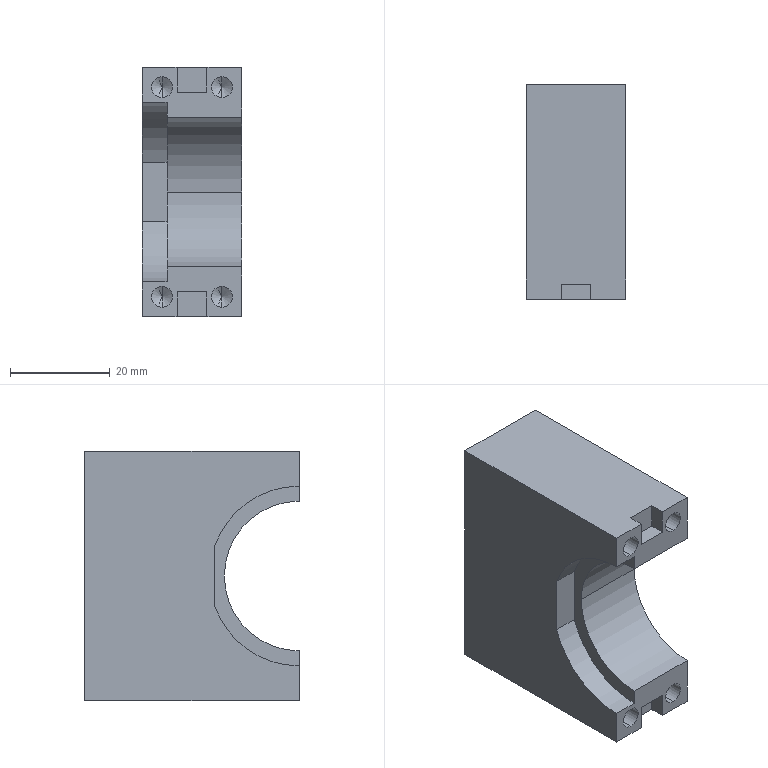Part | SolidWorks | features ICE 4, HoleWzd 2, Extrusion 1 | 1 solid | 50 faces | box 20 x 43 x 50 mm | volume 32312 mm3 | plane 22 | cylinder 16 | cone 12 | commonest cylinder face diameters 4.2 x8 5 x4 30 x2 36 x2
STEP:
#1=CARTESIAN_POINT('',(0.,1.4,10.5));
#2=VERTEX_POINT('',#1);
#3=CARTESIAN_POINT('',(0.,1.4,15.5));
#4=VERTEX_POINT('',#3);
#5=CARTESIAN_POINT('',(0.,1.4,13.));
#6=DIRECTION('',(0.,1.,0.));
#7=DIRECTION('',(0.,0.,1.));
#8=AXIS2_PLACEMENT_3D('',#5,#6,#7);
#9=CIRCLE('',#8,2.5);
#10=EDGE_CURVE('',#2,#4,#9,.T.);
#11=ORIENTED_EDGE('',*,*,#10,.F.);
#12=CARTESIAN_POINT('',(0.,18.5,10.5));
#13=VERTEX_POINT('',#12);
#14=CARTESIAN_POINT('',(0.,18.5,10.5));
#15=DIRECTION('',(0.,1.,0.));
#16=VECTOR('',#15,1000.);
#17=LINE('',#14,#16);
#18=EDGE_CURVE('',#2,#13,#17,.T.);
#19=ORIENTED_EDGE('',*,*,#18,.T.);
#20=CARTESIAN_POINT('',(0.,18.5,15.5));
#21=VERTEX_POINT('',#20);
#22=CARTESIAN_POINT('',(0.,18.5,13.));
#23=DIRECTION('',(0.,1.,0.));
#24=DIRECTION('',(0.,0.,1.));
#25=AXIS2_PLACEMENT_3D('',#22,#23,#24);
#26=CIRCLE('',#25,2.5);
#27=EDGE_CURVE('',#13,#21,#26,.T.);
#28=ORIENTED_EDGE('',*,*,#27,.T.);
#29=CARTESIAN_POINT('',(0.,18.5,15.5));
#30=DIRECTION('',(0.,1.,0.));
#31=VECTOR('',#30,1000.);
#32=LINE('',#29,#31);
#33=EDGE_CURVE('',#4,#21,#32,.T.);
#34=ORIENTED_EDGE('',*,*,#33,.F.);
#35=EDGE_LOOP('',(#11,#19,#28,#34));
#36=FACE_OUTER_BOUND('',#35,.T.);
#37=CARTESIAN_POINT('',(0.,18.5,13.));
#38=DIRECTION('',(0.,1.,0.));
#39=DIRECTION('',(0.,0.,1.));
#40=AXIS2_PLACEMENT_3D('',#37,#38,#39);
#41=CYLINDRICAL_SURFACE('',#40,2.5);
#42=ADVANCED_FACE('',(#36),#41,.F.);
#43=CARTESIAN_POINT('',(0.,-0.1022,13.));
#44=VERTEX_POINT('',#43);
#45=CARTESIAN_POINT('',(0.,1.4,15.5));
#46=DIRECTION('',(0.,0.515,0.8572));
#47=VECTOR('',#46,1000.);
#48=LINE('',#45,#47);
#49=EDGE_CURVE('',#44,#4,#48,.T.);
#50=ORIENTED_EDGE('',*,*,#49,.F.);
#51=CARTESIAN_POINT('',(0.,1.4,10.5));
#52=DIRECTION('',(0.,0.515,-0.8572));
#53=VECTOR('',#52,1000.);
#54=LINE('',#51,#53);
#55=EDGE_CURVE('',#44,#2,#54,.T.);
#56=ORIENTED_EDGE('',*,*,#55,.T.);
#57=ORIENTED_EDGE('',*,*,#10,.T.);
#58=EDGE_LOOP('',(#50,#56,#57));
#59=FACE_OUTER_BOUND('',#58,.T.);
#60=CARTESIAN_POINT('',(0.,1.4,13.));
#61=DIRECTION('',(0.,1.,0.));
#62=DIRECTION('',(0.,0.,1.));
#63=AXIS2_PLACEMENT_3D('',#60,#61,#62);
#64=CONICAL_SURFACE('',#63,2.5,1.03);
#65=ADVANCED_FACE('',(#59),#64,.F.);
#66=CARTESIAN_POINT('',(0.,1.4,34.5));
#67=VERTEX_POINT('',#66);
#68=CARTESIAN_POINT('',(0.,1.4,39.5));
#69=VERTEX_POINT('',#68);
#70=CARTESIAN_POINT('',(0.,1.4,37.));
#71=DIRECTION('',(0.,1.,0.));
#72=DIRECTION('',(0.,0.,1.));
#73=AXIS2_PLACEMENT_3D('',#70,#71,#72);
#74=CIRCLE('',#73,2.5);
#75=EDGE_CURVE('',#67,#69,#74,.T.);
#76=ORIENTED_EDGE('',*,*,#75,.F.);
#77=CARTESIAN_POINT('',(0.,18.5,34.5));
#78=VERTEX_POINT('',#77);
#79=CARTESIAN_POINT('',(0.,18.5,34.5));
#80=DIRECTION('',(0.,1.,0.));
#81=VECTOR('',#80,1000.);
#82=LINE('',#79,#81);
#83=EDGE_CURVE('',#67,#78,#82,.T.);
#84=ORIENTED_EDGE('',*,*,#83,.T.);
#85=CARTESIAN_POINT('',(0.,18.5,39.5));
#86=VERTEX_POINT('',#85);
#87=CARTESIAN_POINT('',(0.,18.5,37.));
#88=DIRECTION('',(0.,1.,0.));
#89=DIRECTION('',(0.,0.,1.));
#90=AXIS2_PLACEMENT_3D('',#87,#88,#89);
#91=CIRCLE('',#90,2.5);
#92=EDGE_CURVE('',#78,#86,#91,.T.);
#93=ORIENTED_EDGE('',*,*,#92,.T.);
#94=CARTESIAN_POINT('',(0.,18.5,39.5));
#95=DIRECTION('',(0.,1.,0.));
#96=VECTOR('',#95,1000.);
#97=LINE('',#94,#96);
#98=EDGE_CURVE('',#69,#86,#97,.T.);
#99=ORIENTED_EDGE('',*,*,#98,.F.);
#100=EDGE_LOOP('',(#76,#84,#93,#99));
#101=FACE_OUTER_BOUND('',#100,.T.);
#102=CARTESIAN_POINT('',(0.,18.5,37.));
#103=DIRECTION('',(0.,1.,0.));
#104=DIRECTION('',(0.,0.,1.));
#105=AXIS2_PLACEMENT_3D('',#102,#103,#104);
#106=CYLINDRICAL_SURFACE('',#105,2.5);
#107=ADVANCED_FACE('',(#101),#106,.F.);
#108=CARTESIAN_POINT('',(0.,-0.1022,37.));
#109=VERTEX_POINT('',#108);
#110=CARTESIAN_POINT('',(0.,1.4,39.5));
#111=DIRECTION('',(0.,0.515,0.8572));
#112=VECTOR('',#111,1000.);
#113=LINE('',#110,#112);
#114=EDGE_CURVE('',#109,#69,#113,.T.);
#115=ORIENTED_EDGE('',*,*,#114,.F.);
#116=CARTESIAN_POINT('',(0.,1.4,34.5));
#117=DIRECTION('',(0.,0.515,-0.8572));
#118=VECTOR('',#117,1000.);
#119=LINE('',#116,#118);
#120=EDGE_CURVE('',#109,#67,#119,.T.);
#121=ORIENTED_EDGE('',*,*,#120,.T.);
#122=ORIENTED_EDGE('',*,*,#75,.T.);
#123=EDGE_LOOP('',(#115,#121,#122));
#124=FACE_OUTER_BOUND('',#123,.T.);
#125=CARTESIAN_POINT('',(0.,1.4,37.));
#126=DIRECTION('',(0.,1.,0.));
#127=DIRECTION('',(0.,0.,1.));
#128=AXIS2_PLACEMENT_3D('',#125,#126,#127);
#129=CONICAL_SURFACE('',#128,2.5,1.03);
#130=ADVANCED_FACE('',(#124),#129,.F.);
#131=CARTESIAN_POINT('',(-6.,-7.3,6.1));
#132=VERTEX_POINT('',#131);
#133=CARTESIAN_POINT('',(-6.,-7.3,1.9));
#134=VERTEX_POINT('',#133);
#135=CARTESIAN_POINT('',(-6.,-7.3,4.));
#136=DIRECTION('',(0.,-1.,0.));
#137=DIRECTION('',(0.,0.,-1.));
#138=AXIS2_PLACEMENT_3D('',#135,#136,#137);
#139=CIRCLE('',#138,2.1);
#140=EDGE_CURVE('',#132,#134,#139,.T.);
#141=ORIENTED_EDGE('',*,*,#140,.F.);
#142=CARTESIAN_POINT('',(-6.,-21.5,6.1));
#143=VERTEX_POINT('',#142);
#144=CARTESIAN_POINT('',(-6.,-21.5,6.1));
#145=DIRECTION('',(0.,-1.,0.));
#146=VECTOR('',#145,1000.);
#147=LINE('',#144,#146);
#148=EDGE_CURVE('',#132,#143,#147,.T.);
#149=ORIENTED_EDGE('',*,*,#148,.T.);
#150=CARTESIAN_POINT('',(-6.,-21.5,1.9));
#151=VERTEX_POINT('',#150);
#152=CARTESIAN_POINT('',(-6.,-21.5,4.));
#153=DIRECTION('',(0.,-1.,0.));
#154=DIRECTION('',(0.,0.,-1.));
#155=AXIS2_PLACEMENT_3D('',#152,#153,#154);
#156=CIRCLE('',#155,2.1);
#157=EDGE_CURVE('',#143,#151,#156,.T.);
#158=ORIENTED_EDGE('',*,*,#157,.T.);
#159=CARTESIAN_POINT('',(-6.,-21.5,1.9));
#160=DIRECTION('',(0.,-1.,0.));
#161=VECTOR('',#160,1000.);
#162=LINE('',#159,#161);
#163=EDGE_CURVE('',#134,#151,#162,.T.);
#164=ORIENTED_EDGE('',*,*,#163,.F.);
#165=EDGE_LOOP('',(#141,#149,#158,#164));
#166=FACE_OUTER_BOUND('',#165,.T.);
#167=CARTESIAN_POINT('',(-6.,-21.5,4.));
#168=DIRECTION('',(0.,-1.,0.));
#169=DIRECTION('',(0.,0.,-1.));
#170=AXIS2_PLACEMENT_3D('',#167,#168,#169);
#171=CYLINDRICAL_SURFACE('',#170,2.1);
#172=ADVANCED_FACE('',(#166),#171,.F.);
#173=CARTESIAN_POINT('',(-6.,-6.038,4.));
#174=VERTEX_POINT('',#173);
#175=CARTESIAN_POINT('',(-6.,-7.3,1.9));
#176=DIRECTION('',(0.,-0.515,-0.8572));
#177=VECTOR('',#176,1000.);
#178=LINE('',#175,#177);
#179=EDGE_CURVE('',#174,#134,#178,.T.);
#180=ORIENTED_EDGE('',*,*,#179,.F.);
#181=CARTESIAN_POINT('',(-6.,-7.3,6.1));
#182=DIRECTION('',(0.,-0.515,0.8572));
#183=VECTOR('',#182,1000.);
#184=LINE('',#181,#183);
#185=EDGE_CURVE('',#174,#132,#184,.T.);
#186=ORIENTED_EDGE('',*,*,#185,.T.);
#187=ORIENTED_EDGE('',*,*,#140,.T.);
#188=EDGE_LOOP('',(#180,#186,#187));
#189=FACE_OUTER_BOUND('',#188,.T.);
#190=CARTESIAN_POINT('',(-6.,-7.3,4.));
#191=DIRECTION('',(0.,-1.,0.));
#192=DIRECTION('',(0.,0.,-1.));
#193=AXIS2_PLACEMENT_3D('',#190,#191,#192);
#194=CONICAL_SURFACE('',#193,2.1,1.03);
#195=ADVANCED_FACE('',(#189),#194,.F.);
#196=CARTESIAN_POINT('',(6.,-7.3,6.1));
#197=VERTEX_POINT('',#196);
#198=CARTESIAN_POINT('',(6.,-7.3,1.9));
#199=VERTEX_POINT('',#198);
#200=CARTESIAN_POINT('',(6.,-7.3,4.));
#201=DIRECTION('',(0.,-1.,0.));
#202=DIRECTION('',(0.,0.,-1.));
#203=AXIS2_PLACEMENT_3D('',#200,#201,#202);
#204=CIRCLE('',#203,2.1);
#205=EDGE_CURVE('',#197,#199,#204,.T.);
#206=ORIENTED_EDGE('',*,*,#205,.F.);
#207=CARTESIAN_POINT('',(6.,-21.5,6.1));
#208=VERTEX_POINT('',#207);
#209=CARTESIAN_POINT('',(6.,-21.5,6.1));
#210=DIRECTION('',(0.,-1.,0.));
#211=VECTOR('',#210,1000.);
#212=LINE('',#209,#211);
#213=EDGE_CURVE('',#197,#208,#212,.T.);
#214=ORIENTED_EDGE('',*,*,#213,.T.);
#215=CARTESIAN_POINT('',(6.,-21.5,1.9));
#216=VERTEX_POINT('',#215);
#217=CARTESIAN_POINT('',(6.,-21.5,4.));
#218=DIRECTION('',(0.,-1.,0.));
#219=DIRECTION('',(0.,0.,-1.));
#220=AXIS2_PLACEMENT_3D('',#217,#218,#219);
#221=CIRCLE('',#220,2.1);
#222=EDGE_CURVE('',#208,#216,#221,.T.);
#223=ORIENTED_EDGE('',*,*,#222,.T.);
#224=CARTESIAN_POINT('',(6.,-21.5,1.9));
#225=DIRECTION('',(0.,-1.,0.));
#226=VECTOR('',#225,1000.);
#227=LINE('',#224,#226);
#228=EDGE_CURVE('',#199,#216,#227,.T.);
#229=ORIENTED_EDGE('',*,*,#228,.F.);
#230=EDGE_LOOP('',(#206,#214,#223,#229));
#231=FACE_OUTER_BOUND('',#230,.T.);
#232=CARTESIAN_POINT('',(6.,-21.5,4.));
#233=DIRECTION('',(0.,-1.,0.));
#234=DIRECTION('',(0.,0.,-1.));
#235=AXIS2_PLACEMENT_3D('',#232,#233,#234);
#236=CYLINDRICAL_SURFACE('',#235,2.1);
#237=ADVANCED_FACE('',(#231),#236,.F.);
#238=CARTESIAN_POINT('',(6.,-6.038,4.));
#239=VERTEX_POINT('',#238);
#240=CARTESIAN_POINT('',(6.,-7.3,1.9));
#241=DIRECTION('',(0.,-0.515,-0.8572));
#242=VECTOR('',#241,1000.);
#243=LINE('',#240,#242);
#244=EDGE_CURVE('',#239,#199,#243,.T.);
#245=ORIENTED_EDGE('',*,*,#244,.F.);
#246=CARTESIAN_POINT('',(6.,-7.3,6.1));
#247=DIRECTION('',(0.,-0.515,0.8572));
#248=VECTOR('',#247,1000.);
#249=LINE('',#246,#248);
#250=EDGE_CURVE('',#239,#197,#249,.T.);
#251=ORIENTED_EDGE('',*,*,#250,.T.);
#252=ORIENTED_EDGE('',*,*,#205,.T.);
#253=EDGE_LOOP('',(#245,#251,#252));
#254=FACE_OUTER_BOUND('',#253,.T.);
#255=CARTESIAN_POINT('',(6.,-7.3,4.));
#256=DIRECTION('',(0.,-1.,0.));
#257=DIRECTION('',(0.,0.,-1.));
#258=AXIS2_PLACEMENT_3D('',#255,#256,#257);
#259=CONICAL_SURFACE('',#258,2.1,1.03);
#260=ADVANCED_FACE('',(#254),#259,.F.);
#261=CARTESIAN_POINT('',(-6.,-7.3,48.1));
#262=VERTEX_POINT('',#261);
#263=CARTESIAN_POINT('',(-6.,-7.3,43.9));
#264=VERTEX_POINT('',#263);
#265=CARTESIAN_POINT('',(-6.,-7.3,46.));
#266=DIRECTION('',(0.,-1.,0.));
#267=DIRECTION('',(0.,0.,-1.));
#268=AXIS2_PLACEMENT_3D('',#265,#266,#267);
#269=CIRCLE('',#268,2.1);
#270=EDGE_CURVE('',#262,#264,#269,.T.);
#271=ORIENTED_EDGE('',*,*,#270,.F.);
#272=CARTESIAN_POINT('',(-6.,-21.5,48.1));
#273=VERTEX_POINT('',#272);
#274=CARTESIAN_POINT('',(-6.,-21.5,48.1));
#275=DIRECTION('',(0.,-1.,0.));
#276=VECTOR('',#275,1000.);
#277=LINE('',#274,#276);
#278=EDGE_CURVE('',#262,#273,#277,.T.);
#279=ORIENTED_EDGE('',*,*,#278,.T.);
#280=CARTESIAN_POINT('',(-6.,-21.5,43.9));
#281=VERTEX_POINT('',#280);
#282=CARTESIAN_POINT('',(-6.,-21.5,46.));
#283=DIRECTION('',(0.,-1.,0.));
#284=DIRECTION('',(0.,0.,-1.));
#285=AXIS2_PLACEMENT_3D('',#282,#283,#284);
#286=CIRCLE('',#285,2.1);
#287=EDGE_CURVE('',#273,#281,#286,.T.);
#288=ORIENTED_EDGE('',*,*,#287,.T.);
#289=CARTESIAN_POINT('',(-6.,-21.5,43.9));
#290=DIRECTION('',(0.,-1.,0.));
#291=VECTOR('',#290,1000.);
#292=LINE('',#289,#291);
#293=EDGE_CURVE('',#264,#281,#292,.T.);
#294=ORIENTED_EDGE('',*,*,#293,.F.);
#295=EDGE_LOOP('',(#271,#279,#288,#294));
#296=FACE_OUTER_BOUND('',#295,.T.);
#297=CARTESIAN_POINT('',(-6.,-21.5,46.));
#298=DIRECTION('',(0.,-1.,0.));
#299=DIRECTION('',(0.,0.,-1.));
#300=AXIS2_PLACEMENT_3D('',#297,#298,#299);
#301=CYLINDRICAL_SURFACE('',#300,2.1);
#302=ADVANCED_FACE('',(#296),#301,.F.);
#303=CARTESIAN_POINT('',(-6.,-6.038,46.));
#304=VERTEX_POINT('',#303);
#305=CARTESIAN_POINT('',(-6.,-7.3,43.9));
#306=DIRECTION('',(0.,-0.515,-0.8572));
#307=VECTOR('',#306,1000.);
#308=LINE('',#305,#307);
#309=EDGE_CURVE('',#304,#264,#308,.T.);
#310=ORIENTED_EDGE('',*,*,#309,.F.);
#311=CARTESIAN_POINT('',(-6.,-7.3,48.1));
#312=DIRECTION('',(0.,-0.515,0.8572));
#313=VECTOR('',#312,1000.);
#314=LINE('',#311,#313);
#315=EDGE_CURVE('',#304,#262,#314,.T.);
#316=ORIENTED_EDGE('',*,*,#315,.T.);
#317=ORIENTED_EDGE('',*,*,#270,.T.);
#318=EDGE_LOOP('',(#310,#316,#317));
#319=FACE_OUTER_BOUND('',#318,.T.);
#320=CARTESIAN_POINT('',(-6.,-7.3,46.));
#321=DIRECTION('',(0.,-1.,0.));
#322=DIRECTION('',(0.,0.,-1.));
#323=AXIS2_PLACEMENT_3D('',#320,#321,#322);
#324=CONICAL_SURFACE('',#323,2.1,1.03);
#325=ADVANCED_FACE('',(#319),#324,.F.);
#326=CARTESIAN_POINT('',(6.,-7.3,48.1));
#327=VERTEX_POINT('',#326);
#328=CARTESIAN_POINT('',(6.,-7.3,43.9));
#329=VERTEX_POINT('',#328);
#330=CARTESIAN_POINT('',(6.,-7.3,46.));
#331=DIRECTION('',(0.,-1.,0.));
#332=DIRECTION('',(0.,0.,-1.));
#333=AXIS2_PLACEMENT_3D('',#330,#331,#332);
#334=CIRCLE('',#333,2.1);
#335=EDGE_CURVE('',#327,#329,#334,.T.);
#336=ORIENTED_EDGE('',*,*,#335,.F.);
#337=CARTESIAN_POINT('',(6.,-21.5,48.1));
#338=VERTEX_POINT('',#337);
#339=CARTESIAN_POINT('',(6.,-21.5,48.1));
#340=DIRECTION('',(0.,-1.,0.));
#341=VECTOR('',#340,1000.);
#342=LINE('',#339,#341);
#343=EDGE_CURVE('',#327,#338,#342,.T.);
#344=ORIENTED_EDGE('',*,*,#343,.T.);
#345=CARTESIAN_POINT('',(6.,-21.5,43.9));
#346=VERTEX_POINT('',#345);
#347=CARTESIAN_POINT('',(6.,-21.5,46.));
#348=DIRECTION('',(0.,-1.,0.));
#349=DIRECTION('',(0.,0.,-1.));
#350=AXIS2_PLACEMENT_3D('',#347,#348,#349);
#351=CIRCLE('',#350,2.1);
#352=EDGE_CURVE('',#338,#346,#351,.T.);
#353=ORIENTED_EDGE('',*,*,#352,.T.);
#354=CARTESIAN_POINT('',(6.,-21.5,43.9));
#355=DIRECTION('',(0.,-1.,0.));
#356=VECTOR('',#355,1000.);
#357=LINE('',#354,#356);
#358=EDGE_CURVE('',#329,#346,#357,.T.);
#359=ORIENTED_EDGE('',*,*,#358,.F.);
#360=EDGE_LOOP('',(#336,#344,#353,#359));
#361=FACE_OUTER_BOUND('',#360,.T.);
#362=CARTESIAN_POINT('',(6.,-21.5,46.));
#363=DIRECTION('',(0.,-1.,0.));
#364=DIRECTION('',(0.,0.,-1.));
#365=AXIS2_PLACEMENT_3D('',#362,#363,#364);
#366=CYLINDRICAL_SURFACE('',#365,2.1);
#367=ADVANCED_FACE('',(#361),#366,.F.);
#368=CARTESIAN_POINT('',(6.,-6.038,46.));
#369=VERTEX_POINT('',#368);
#370=CARTESIAN_POINT('',(6.,-7.3,43.9));
#371=DIRECTION('',(0.,-0.515,-0.8572));
#372=VECTOR('',#371,1000.);
#373=LINE('',#370,#372);
#374=EDGE_CURVE('',#369,#329,#373,.T.);
#375=ORIENTED_EDGE('',*,*,#374,.F.);
#376=CARTESIAN_POINT('',(6.,-7.3,48.1));
#377=DIRECTION('',(0.,-0.515,0.8572));
#378=VECTOR('',#377,1000.);
#379=LINE('',#376,#378);
#380=EDGE_CURVE('',#369,#327,#379,.T.);
#381=ORIENTED_EDGE('',*,*,#380,.T.);
#382=ORIENTED_EDGE('',*,*,#335,.T.);
#383=EDGE_LOOP('',(#375,#381,#382));
#384=FACE_OUTER_BOUND('',#383,.T.);
#385=CARTESIAN_POINT('',(6.,-7.3,46.));
#386=DIRECTION('',(0.,-1.,0.));
#387=DIRECTION('',(0.,0.,-1.));
#388=AXIS2_PLACEMENT_3D('',#385,#386,#387);
#389=CONICAL_SURFACE('',#388,2.1,1.03);
#390=ADVANCED_FACE('',(#384),#389,.F.);
#391=CARTESIAN_POINT('',(-5.,-6.5,25.));
#392=VERTEX_POINT('',#391);
#393=CARTESIAN_POINT('',(-5.,-21.5,40.));
#394=VERTEX_POINT('',#393);
#395=CARTESIAN_POINT('',(-5.,-21.5,25.));
#396=DIRECTION('',(1.,0.,0.));
#397=DIRECTION('',(0.,-1.,0.));
#398=AXIS2_PLACEMENT_3D('',#395,#396,#397);
#399=CIRCLE('',#398,15.);
#400=EDGE_CURVE('',#392,#394,#399,.T.);
#401=ORIENTED_EDGE('',*,*,#400,.F.);
#402=CARTESIAN_POINT('',(10.,-6.5,25.));
#403=VERTEX_POINT('',#402);
#404=CARTESIAN_POINT('',(-40.,-6.5,25.));
#405=DIRECTION('',(1.,0.,0.));
#406=VECTOR('',#405,1000.);
#407=LINE('',#404,#406);
#408=EDGE_CURVE('',#392,#403,#407,.T.);
#409=ORIENTED_EDGE('',*,*,#408,.T.);
#410=CARTESIAN_POINT('',(10.,-21.5,40.));
#411=VERTEX_POINT('',#410);
#412=CARTESIAN_POINT('',(10.,-21.5,25.));
#413=DIRECTION('',(-1.,0.,0.));
#414=DIRECTION('',(0.,-1.,0.));
#415=AXIS2_PLACEMENT_3D('',#412,#413,#414);
#416=CIRCLE('',#415,15.);
#417=EDGE_CURVE('',#411,#403,#416,.T.);
#418=ORIENTED_EDGE('',*,*,#417,.F.);
#419=CARTESIAN_POINT('',(-40.,-21.5,40.));
#420=DIRECTION('',(1.,0.,0.));
#421=VECTOR('',#420,1000.);
#422=LINE('',#419,#421);
#423=EDGE_CURVE('',#394,#411,#422,.T.);
#424=ORIENTED_EDGE('',*,*,#423,.F.);
#425=EDGE_LOOP('',(#401,#409,#418,#424));
#426=FACE_OUTER_BOUND('',#425,.T.);
#427=CARTESIAN_POINT('',(-40.,-21.5,25.));
#428=DIRECTION('',(1.,0.,0.));
#429=DIRECTION('',(0.,1.,0.));
#430=AXIS2_PLACEMENT_3D('',#427,#428,#429);
#431=CYLINDRICAL_SURFACE('',#430,15.);
#432=ADVANCED_FACE('',(#426),#431,.F.);
#433=ORIENTED_EDGE('',*,*,#408,.F.);
#434=CARTESIAN_POINT('',(-5.,-21.5,10.));
#435=VERTEX_POINT('',#434);
#436=CARTESIAN_POINT('',(-5.,-21.5,25.));
#437=DIRECTION('',(1.,0.,0.));
#438=DIRECTION('',(0.,-1.,0.));
#439=AXIS2_PLACEMENT_3D('',#436,#437,#438);
#440=CIRCLE('',#439,15.);
#441=EDGE_CURVE('',#435,#392,#440,.T.);
#442=ORIENTED_EDGE('',*,*,#441,.F.);
#443=CARTESIAN_POINT('',(10.,-21.5,10.));
#444=VERTEX_POINT('',#443);
#445=CARTESIAN_POINT('',(-40.,-21.5,10.));
#446=DIRECTION('',(-1.,0.,0.));
#447=VECTOR('',#446,1000.);
#448=LINE('',#445,#447);
#449=EDGE_CURVE('',#444,#435,#448,.T.);
#450=ORIENTED_EDGE('',*,*,#449,.F.);
#451=CARTESIAN_POINT('',(10.,-21.5,25.));
#452=DIRECTION('',(-1.,0.,0.));
#453=DIRECTION('',(0.,-1.,0.));
#454=AXIS2_PLACEMENT_3D('',#451,#452,#453);
#455=CIRCLE('',#454,15.);
#456=EDGE_CURVE('',#403,#444,#455,.T.);
#457=ORIENTED_EDGE('',*,*,#456,.F.);
#458=EDGE_LOOP('',(#433,#442,#450,#457));
#459=FACE_OUTER_BOUND('',#458,.T.);
#460=CARTESIAN_POINT('',(-40.,-21.5,25.));
#461=DIRECTION('',(1.,0.,0.));
#462=DIRECTION('',(0.,1.,0.));
#463=AXIS2_PLACEMENT_3D('',#460,#461,#462);
#464=CYLINDRICAL_SURFACE('',#463,15.);
#465=ADVANCED_FACE('',(#459),#464,.F.);
#466=CARTESIAN_POINT('',(-6.,-21.5,46.));
#467=DIRECTION('',(0.,-1.,0.));
#468=DIRECTION('',(0.,0.,-1.));
#469=AXIS2_PLACEMENT_3D('',#466,#467,#468);
#470=CIRCLE('',#469,2.1);
#471=EDGE_CURVE('',#281,#273,#470,.T.);
#472=ORIENTED_EDGE('',*,*,#471,.F.);
#473=ORIENTED_EDGE('',*,*,#287,.F.);
#474=EDGE_LOOP('',(#472,#473));
#475=FACE_BOUND('',#474,.T.);
#476=CARTESIAN_POINT('',(6.,-21.5,46.));
#477=DIRECTION('',(0.,-1.,0.));
#478=DIRECTION('',(0.,0.,-1.));
#479=AXIS2_PLACEMENT_3D('',#476,#477,#478);
#480=CIRCLE('',#479,2.1);
#481=EDGE_CURVE('',#346,#338,#480,.T.);
#482=ORIENTED_EDGE('',*,*,#481,.F.);
#483=ORIENTED_EDGE('',*,*,#352,.F.);
#484=EDGE_LOOP('',(#482,#483));
#485=FACE_BOUND('',#484,.T.);
#486=CARTESIAN_POINT('',(-3.,-21.5,45.));
#487=VERTEX_POINT('',#486);
#488=CARTESIAN_POINT('',(3.,-21.5,45.));
#489=VERTEX_POINT('',#488);
#490=CARTESIAN_POINT('',(-3.,-21.5,45.));
#491=DIRECTION('',(1.,0.,0.));
#492=VECTOR('',#491,1000.);
#493=LINE('',#490,#492);
#494=EDGE_CURVE('',#487,#489,#493,.T.);
#495=ORIENTED_EDGE('',*,*,#494,.F.);
#496=CARTESIAN_POINT('',(-3.,-21.5,50.));
#497=VERTEX_POINT('',#496);
#498=CARTESIAN_POINT('',(-3.,-21.5,45.));
#499=DIRECTION('',(0.,0.,-1.));
#500=VECTOR('',#499,1000.);
#501=LINE('',#498,#500);
#502=EDGE_CURVE('',#497,#487,#501,.T.);
#503=ORIENTED_EDGE('',*,*,#502,.F.);
#504=CARTESIAN_POINT('',(-10.,-21.5,50.));
#505=VERTEX_POINT('',#504);
#506=CARTESIAN_POINT('',(10.,-21.5,50.));
#507=DIRECTION('',(1.,0.,0.));
#508=VECTOR('',#507,1000.);
#509=LINE('',#506,#508);
#510=EDGE_CURVE('',#505,#497,#509,.T.);
#511=ORIENTED_EDGE('',*,*,#510,.F.);
#512=CARTESIAN_POINT('',(-10.,-21.5,43.));
#513=VERTEX_POINT('',#512);
#514=CARTESIAN_POINT('',(-10.,-21.5,50.));
#515=DIRECTION('',(0.,0.,-1.));
#516=VECTOR('',#515,1000.);
#517=LINE('',#514,#516);
#518=EDGE_CURVE('',#505,#513,#517,.T.);
#519=ORIENTED_EDGE('',*,*,#518,.T.);
#520=CARTESIAN_POINT('',(-5.,-21.5,43.));
#521=VERTEX_POINT('',#520);
#522=CARTESIAN_POINT('',(-5.,-21.5,43.));
#523=DIRECTION('',(1.,0.,0.));
#524=VECTOR('',#523,1000.);
#525=LINE('',#522,#524);
#526=EDGE_CURVE('',#513,#521,#525,.T.);
#527=ORIENTED_EDGE('',*,*,#526,.T.);
#528=CARTESIAN_POINT('',(-5.,-21.5,50.));
#529=DIRECTION('',(0.,0.,1.));
#530=VECTOR('',#529,1000.);
#531=LINE('',#528,#530);
#532=EDGE_CURVE('',#394,#521,#531,.T.);
#533=ORIENTED_EDGE('',*,*,#532,.F.);
#534=ORIENTED_EDGE('',*,*,#423,.T.);
#535=CARTESIAN_POINT('',(10.,-21.5,50.));
#536=VERTEX_POINT('',#535);
#537=CARTESIAN_POINT('',(10.,-21.5,50.));
#538=DIRECTION('',(0.,0.,-1.));
#539=VECTOR('',#538,1000.);
#540=LINE('',#537,#539);
#541=EDGE_CURVE('',#536,#411,#540,.T.);
#542=ORIENTED_EDGE('',*,*,#541,.F.);
#543=CARTESIAN_POINT('',(3.,-21.5,50.));
#544=VERTEX_POINT('',#543);
#545=CARTESIAN_POINT('',(10.,-21.5,50.));
#546=DIRECTION('',(1.,0.,0.));
#547=VECTOR('',#546,1000.);
#548=LINE('',#545,#547);
#549=EDGE_CURVE('',#544,#536,#548,.T.);
#550=ORIENTED_EDGE('',*,*,#549,.F.);
#551=CARTESIAN_POINT('',(3.,-21.5,45.));
#552=DIRECTION('',(0.,0.,1.));
#553=VECTOR('',#552,1000.);
#554=LINE('',#551,#553);
#555=EDGE_CURVE('',#489,#544,#554,.T.);
#556=ORIENTED_EDGE('',*,*,#555,.F.);
#557=EDGE_LOOP('',(#495,#503,#511,#519,#527,#533,#534,#542,#550,#556));
#558=FACE_OUTER_BOUND('',#557,.T.);
#559=CARTESIAN_POINT('',(10.,-21.5,50.));
#560=DIRECTION('',(0.,1.,0.));
#561=DIRECTION('',(0.,0.,1.));
#562=AXIS2_PLACEMENT_3D('',#559,#560,#561);
#563=PLANE('',#562);
#564=ADVANCED_FACE('',(#475,#485,#558),#563,.F.);
#565=CARTESIAN_POINT('',(-10.,-4.5,30.916));
#566=VERTEX_POINT('',#565);
#567=CARTESIAN_POINT('',(-10.,-4.5,19.084));
#568=VERTEX_POINT('',#567);
#569=CARTESIAN_POINT('',(-10.,-4.5,19.084));
#570=DIRECTION('',(0.,0.,-1.));
#571=VECTOR('',#570,1000.);
#572=LINE('',#569,#571);
#573=EDGE_CURVE('',#566,#568,#572,.T.);
#574=ORIENTED_EDGE('',*,*,#573,.F.);
#575=CARTESIAN_POINT('',(-10.,-21.5,25.));
#576=DIRECTION('',(-1.,0.,0.));
#577=DIRECTION('',(0.,-1.,0.));
#578=AXIS2_PLACEMENT_3D('',#575,#576,#577);
#579=CIRCLE('',#578,18.);
#580=EDGE_CURVE('',#513,#566,#579,.T.);
#581=ORIENTED_EDGE('',*,*,#580,.F.);
#582=ORIENTED_EDGE('',*,*,#518,.F.);
#583=CARTESIAN_POINT('',(-10.,21.5,50.));
#584=VERTEX_POINT('',#583);
#585=CARTESIAN_POINT('',(-10.,21.5,50.));
#586=DIRECTION('',(0.,-1.,0.));
#587=VECTOR('',#586,1000.);
#588=LINE('',#585,#587);
#589=EDGE_CURVE('',#584,#505,#588,.T.);
#590=ORIENTED_EDGE('',*,*,#589,.F.);
#591=CARTESIAN_POINT('',(-10.,21.5,0.));
#592=VERTEX_POINT('',#591);
#593=CARTESIAN_POINT('',(-10.,21.5,50.));
#594=DIRECTION('',(0.,0.,-1.));
#595=VECTOR('',#594,1000.);
#596=LINE('',#593,#595);
#597=EDGE_CURVE('',#584,#592,#596,.T.);
#598=ORIENTED_EDGE('',*,*,#597,.T.);
#599=CARTESIAN_POINT('',(-10.,-21.5,0.));
#600=VERTEX_POINT('',#599);
#601=CARTESIAN_POINT('',(-10.,21.5,0.));
#602=DIRECTION('',(0.,-1.,0.));
#603=VECTOR('',#602,1000.);
#604=LINE('',#601,#603);
#605=EDGE_CURVE('',#592,#600,#604,.T.);
#606=ORIENTED_EDGE('',*,*,#605,.T.);
#607=CARTESIAN_POINT('',(-10.,-21.5,7.));
#608=VERTEX_POINT('',#607);
#609=CARTESIAN_POINT('',(-10.,-21.5,50.));
#610=DIRECTION('',(0.,0.,-1.));
#611=VECTOR('',#610,1000.);
#612=LINE('',#609,#611);
#613=EDGE_CURVE('',#608,#600,#612,.T.);
#614=ORIENTED_EDGE('',*,*,#613,.F.);
#615=CARTESIAN_POINT('',(-10.,-21.5,25.));
#616=DIRECTION('',(-1.,0.,0.));
#617=DIRECTION('',(0.,-1.,0.));
#618=AXIS2_PLACEMENT_3D('',#615,#616,#617);
#619=CIRCLE('',#618,18.);
#620=EDGE_CURVE('',#568,#608,#619,.T.);
#621=ORIENTED_EDGE('',*,*,#620,.F.);
#622=EDGE_LOOP('',(#574,#581,#582,#590,#598,#606,#614,#621));
#623=FACE_OUTER_BOUND('',#622,.T.);
#624=CARTESIAN_POINT('',(-10.,21.5,50.));
#625=DIRECTION('',(1.,0.,0.));
#626=DIRECTION('',(0.,1.,0.));
#627=AXIS2_PLACEMENT_3D('',#624,#625,#626);
#628=PLANE('',#627);
#629=ADVANCED_FACE('',(#623),#628,.F.);
#630=CARTESIAN_POINT('',(-6.,-21.5,4.));
#631=DIRECTION('',(0.,-1.,0.));
#632=DIRECTION('',(0.,0.,-1.));
#633=AXIS2_PLACEMENT_3D('',#630,#631,#632);
#634=CIRCLE('',#633,2.1);
#635=EDGE_CURVE('',#151,#143,#634,.T.);
#636=ORIENTED_EDGE('',*,*,#635,.F.);
#637=ORIENTED_EDGE('',*,*,#157,.F.);
#638=EDGE_LOOP('',(#636,#637));
#639=FACE_BOUND('',#638,.T.);
#640=CARTESIAN_POINT('',(6.,-21.5,4.));
#641=DIRECTION('',(0.,-1.,0.));
#642=DIRECTION('',(0.,0.,-1.));
#643=AXIS2_PLACEMENT_3D('',#640,#641,#642);
#644=CIRCLE('',#643,2.1);
#645=EDGE_CURVE('',#216,#208,#644,.T.);
#646=ORIENTED_EDGE('',*,*,#645,.F.);
#647=ORIENTED_EDGE('',*,*,#222,.F.);
#648=EDGE_LOOP('',(#646,#647));
#649=FACE_BOUND('',#648,.T.);
#650=CARTESIAN_POINT('',(3.,-21.5,5.));
#651=VERTEX_POINT('',#650);
#652=CARTESIAN_POINT('',(-3.,-21.5,5.));
#653=VERTEX_POINT('',#652);
#654=CARTESIAN_POINT('',(-3.,-21.5,5.));
#655=DIRECTION('',(-1.,0.,0.));
#656=VECTOR('',#655,1000.);
#657=LINE('',#654,#656);
#658=EDGE_CURVE('',#651,#653,#657,.T.);
#659=ORIENTED_EDGE('',*,*,#658,.F.);
#660=CARTESIAN_POINT('',(3.,-21.5,0.));
#661=VERTEX_POINT('',#660);
#662=CARTESIAN_POINT('',(3.,-21.5,5.));
#663=DIRECTION('',(0.,0.,1.));
#664=VECTOR('',#663,1000.);
#665=LINE('',#662,#664);
#666=EDGE_CURVE('',#661,#651,#665,.T.);
#667=ORIENTED_EDGE('',*,*,#666,.F.);
#668=CARTESIAN_POINT('',(10.,-21.5,0.));
#669=VERTEX_POINT('',#668);
#670=CARTESIAN_POINT('',(10.,-21.5,0.));
#671=DIRECTION('',(1.,0.,0.));
#672=VECTOR('',#671,1000.);
#673=LINE('',#670,#672);
#674=EDGE_CURVE('',#661,#669,#673,.T.);
#675=ORIENTED_EDGE('',*,*,#674,.T.);
#676=CARTESIAN_POINT('',(10.,-21.5,50.));
#677=DIRECTION('',(0.,0.,-1.));
#678=VECTOR('',#677,1000.);
#679=LINE('',#676,#678);
#680=EDGE_CURVE('',#444,#669,#679,.T.);
#681=ORIENTED_EDGE('',*,*,#680,.F.);
#682=ORIENTED_EDGE('',*,*,#449,.T.);
#683=CARTESIAN_POINT('',(-5.,-21.5,7.));
#684=VERTEX_POINT('',#683);
#685=CARTESIAN_POINT('',(-5.,-21.5,50.));
#686=DIRECTION('',(0.,0.,1.));
#687=VECTOR('',#686,1000.);
#688=LINE('',#685,#687);
#689=EDGE_CURVE('',#684,#435,#688,.T.);
#690=ORIENTED_EDGE('',*,*,#689,.F.);
#691=CARTESIAN_POINT('',(-5.,-21.5,7.));
#692=DIRECTION('',(-1.,0.,0.));
#693=VECTOR('',#692,1000.);
#694=LINE('',#691,#693);
#695=EDGE_CURVE('',#684,#608,#694,.T.);
#696=ORIENTED_EDGE('',*,*,#695,.T.);
#697=ORIENTED_EDGE('',*,*,#613,.T.);
#698=CARTESIAN_POINT('',(-3.,-21.5,0.));
#699=VERTEX_POINT('',#698);
#700=CARTESIAN_POINT('',(10.,-21.5,0.));
#701=DIRECTION('',(1.,0.,0.));
#702=VECTOR('',#701,1000.);
#703=LINE('',#700,#702);
#704=EDGE_CURVE('',#600,#699,#703,.T.);
#705=ORIENTED_EDGE('',*,*,#704,.T.);
#706=CARTESIAN_POINT('',(-3.,-21.5,5.));
#707=DIRECTION('',(0.,0.,-1.));
#708=VECTOR('',#707,1000.);
#709=LINE('',#706,#708);
#710=EDGE_CURVE('',#653,#699,#709,.T.);
#711=ORIENTED_EDGE('',*,*,#710,.F.);
#712=EDGE_LOOP('',(#659,#667,#675,#681,#682,#690,#696,#697,#705,#711));
#713=FACE_OUTER_BOUND('',#712,.T.);
#714=CARTESIAN_POINT('',(10.,-21.5,50.));
#715=DIRECTION('',(0.,1.,0.));
#716=DIRECTION('',(0.,0.,1.));
#717=AXIS2_PLACEMENT_3D('',#714,#715,#716);
#718=PLANE('',#717);
#719=ADVANCED_FACE('',(#639,#649,#713),#718,.F.);
#720=ORIENTED_EDGE('',*,*,#541,.T.);
#721=ORIENTED_EDGE('',*,*,#417,.T.);
#722=ORIENTED_EDGE('',*,*,#456,.T.);
#723=ORIENTED_EDGE('',*,*,#680,.T.);
#724=CARTESIAN_POINT('',(10.,21.5,0.));
#725=VERTEX_POINT('',#724);
#726=CARTESIAN_POINT('',(10.,21.5,0.));
#727=DIRECTION('',(0.,1.,0.));
#728=VECTOR('',#727,1000.);
#729=LINE('',#726,#728);
#730=EDGE_CURVE('',#669,#725,#729,.T.);
#731=ORIENTED_EDGE('',*,*,#730,.T.);
#732=CARTESIAN_POINT('',(10.,21.5,50.));
#733=VERTEX_POINT('',#732);
#734=CARTESIAN_POINT('',(10.,21.5,50.));
#735=DIRECTION('',(0.,0.,-1.));
#736=VECTOR('',#735,1000.);
#737=LINE('',#734,#736);
#738=EDGE_CURVE('',#733,#725,#737,.T.);
#739=ORIENTED_EDGE('',*,*,#738,.F.);
#740=CARTESIAN_POINT('',(10.,21.5,50.));
#741=DIRECTION('',(0.,1.,0.));
#742=VECTOR('',#741,1000.);
#743=LINE('',#740,#742);
#744=EDGE_CURVE('',#536,#733,#743,.T.);
#745=ORIENTED_EDGE('',*,*,#744,.F.);
#746=EDGE_LOOP('',(#720,#721,#722,#723,#731,#739,#745));
#747=FACE_OUTER_BOUND('',#746,.T.);
#748=CARTESIAN_POINT('',(10.,21.5,50.));
#749=DIRECTION('',(-1.,0.,0.));
#750=DIRECTION('',(0.,-1.,0.));
#751=AXIS2_PLACEMENT_3D('',#748,#749,#750);
#752=PLANE('',#751);
#753=ADVANCED_FACE('',(#747),#752,.F.);
#754=CARTESIAN_POINT('',(-5.,21.5,45.));
#755=VERTEX_POINT('',#754);
#756=CARTESIAN_POINT('',(5.,21.5,45.));
#757=VERTEX_POINT('',#756);
#758=CARTESIAN_POINT('',(5.,21.5,45.));
#759=DIRECTION('',(1.,0.,0.));
#760=VECTOR('',#759,1000.);
#761=LINE('',#758,#760);
#762=EDGE_CURVE('',#755,#757,#761,.T.);
#763=ORIENTED_EDGE('',*,*,#762,.F.);
#764=CARTESIAN_POINT('',(-5.,21.5,5.));
#765=VERTEX_POINT('',#764);
#766=CARTESIAN_POINT('',(-5.,21.5,45.));
#767=DIRECTION('',(0.,0.,1.));
#768=VECTOR('',#767,1000.);
#769=LINE('',#766,#768);
#770=EDGE_CURVE('',#765,#755,#769,.T.);
#771=ORIENTED_EDGE('',*,*,#770,.F.);
#772=CARTESIAN_POINT('',(5.,21.5,5.));
#773=VERTEX_POINT('',#772);
#774=CARTESIAN_POINT('',(5.,21.5,5.));
#775=DIRECTION('',(-1.,0.,0.));
#776=VECTOR('',#775,1000.);
#777=LINE('',#774,#776);
#778=EDGE_CURVE('',#773,#765,#777,.T.);
#779=ORIENTED_EDGE('',*,*,#778,.F.);
#780=CARTESIAN_POINT('',(5.,21.5,45.));
#781=DIRECTION('',(0.,0.,-1.));
#782=VECTOR('',#781,1000.);
#783=LINE('',#780,#782);
#784=EDGE_CURVE('',#757,#773,#783,.T.);
#785=ORIENTED_EDGE('',*,*,#784,.F.);
#786=EDGE_LOOP('',(#763,#771,#779,#785));
#787=FACE_BOUND('',#786,.T.);
#788=CARTESIAN_POINT('',(10.,21.5,0.));
#789=DIRECTION('',(-1.,0.,0.));
#790=VECTOR('',#789,1000.);
#791=LINE('',#788,#790);
#792=EDGE_CURVE('',#725,#592,#791,.T.);
#793=ORIENTED_EDGE('',*,*,#792,.T.);
#794=ORIENTED_EDGE('',*,*,#597,.F.);
#795=CARTESIAN_POINT('',(10.,21.5,50.));
#796=DIRECTION('',(-1.,0.,0.));
#797=VECTOR('',#796,1000.);
#798=LINE('',#795,#797);
#799=EDGE_CURVE('',#733,#584,#798,.T.);
#800=ORIENTED_EDGE('',*,*,#799,.F.);
#801=ORIENTED_EDGE('',*,*,#738,.T.);
#802=EDGE_LOOP('',(#793,#794,#800,#801));
#803=FACE_OUTER_BOUND('',#802,.T.);
#804=CARTESIAN_POINT('',(10.,21.5,50.));
#805=DIRECTION('',(0.,-1.,0.));
#806=DIRECTION('',(0.,0.,-1.));
#807=AXIS2_PLACEMENT_3D('',#804,#805,#806);
#808=PLANE('',#807);
#809=ADVANCED_FACE('',(#787,#803),#808,.F.);
#810=ORIENTED_EDGE('',*,*,#510,.T.);
#811=CARTESIAN_POINT('',(-3.,-18.5,50.));
#812=VERTEX_POINT('',#811);
#813=CARTESIAN_POINT('',(-3.,-18.5,50.));
#814=DIRECTION('',(0.,-1.,0.));
#815=VECTOR('',#814,1000.);
#816=LINE('',#813,#815);
#817=EDGE_CURVE('',#812,#497,#816,.T.);
#818=ORIENTED_EDGE('',*,*,#817,.F.);
#819=CARTESIAN_POINT('',(3.,-18.5,50.));
#820=VERTEX_POINT('',#819);
#821=CARTESIAN_POINT('',(-3.,-18.5,50.));
#822=DIRECTION('',(-1.,0.,0.));
#823=VECTOR('',#822,1000.);
#824=LINE('',#821,#823);
#825=EDGE_CURVE('',#820,#812,#824,.T.);
#826=ORIENTED_EDGE('',*,*,#825,.F.);
#827=CARTESIAN_POINT('',(3.,-18.5,50.));
#828=DIRECTION('',(0.,-1.,0.));
#829=VECTOR('',#828,1000.);
#830=LINE('',#827,#829);
#831=EDGE_CURVE('',#820,#544,#830,.T.);
#832=ORIENTED_EDGE('',*,*,#831,.T.);
#833=ORIENTED_EDGE('',*,*,#549,.T.);
#834=ORIENTED_EDGE('',*,*,#744,.T.);
#835=ORIENTED_EDGE('',*,*,#799,.T.);
#836=ORIENTED_EDGE('',*,*,#589,.T.);
#837=EDGE_LOOP('',(#810,#818,#826,#832,#833,#834,#835,#836));
#838=FACE_OUTER_BOUND('',#837,.T.);
#839=CARTESIAN_POINT('',(0.,0.,50.));
#840=DIRECTION('',(0.,0.,-1.));
#841=DIRECTION('',(-1.,0.,0.));
#842=AXIS2_PLACEMENT_3D('',#839,#840,#841);
#843=PLANE('',#842);
#844=ADVANCED_FACE('',(#838),#843,.F.);
#845=CARTESIAN_POINT('',(3.,-18.5,0.));
#846=VERTEX_POINT('',#845);
#847=CARTESIAN_POINT('',(3.,-18.5,0.));
#848=DIRECTION('',(0.,-1.,0.));
#849=VECTOR('',#848,1000.);
#850=LINE('',#847,#849);
#851=EDGE_CURVE('',#846,#661,#850,.T.);
#852=ORIENTED_EDGE('',*,*,#851,.F.);
#853=CARTESIAN_POINT('',(-3.,-18.5,0.));
#854=VERTEX_POINT('',#853);
#855=CARTESIAN_POINT('',(-3.,-18.5,0.));
#856=DIRECTION('',(1.,0.,0.));
#857=VECTOR('',#856,1000.);
#858=LINE('',#855,#857);
#859=EDGE_CURVE('',#854,#846,#858,.T.);
#860=ORIENTED_EDGE('',*,*,#859,.F.);
#861=CARTESIAN_POINT('',(-3.,-18.5,0.));
#862=DIRECTION('',(0.,-1.,0.));
#863=VECTOR('',#862,1000.);
#864=LINE('',#861,#863);
#865=EDGE_CURVE('',#854,#699,#864,.T.);
#866=ORIENTED_EDGE('',*,*,#865,.T.);
#867=ORIENTED_EDGE('',*,*,#704,.F.);
#868=ORIENTED_EDGE('',*,*,#605,.F.);
#869=ORIENTED_EDGE('',*,*,#792,.F.);
#870=ORIENTED_EDGE('',*,*,#730,.F.);
#871=ORIENTED_EDGE('',*,*,#674,.F.);
#872=EDGE_LOOP('',(#852,#860,#866,#867,#868,#869,#870,#871));
#873=FACE_OUTER_BOUND('',#872,.T.);
#874=CARTESIAN_POINT('',(0.,0.,0.));
#875=DIRECTION('',(0.,0.,-1.));
#876=DIRECTION('',(-1.,0.,0.));
#877=AXIS2_PLACEMENT_3D('',#874,#875,#876);
#878=PLANE('',#877);
#879=ADVANCED_FACE('',(#873),#878,.T.);
#880=ORIENTED_EDGE('',*,*,#580,.T.);
#881=CARTESIAN_POINT('',(-5.,-4.5,30.916));
#882=VERTEX_POINT('',#881);
#883=CARTESIAN_POINT('',(-5.,-4.5,30.916));
#884=DIRECTION('',(-1.,0.,0.));
#885=VECTOR('',#884,1000.);
#886=LINE('',#883,#885);
#887=EDGE_CURVE('',#882,#566,#886,.T.);
#888=ORIENTED_EDGE('',*,*,#887,.F.);
#889=CARTESIAN_POINT('',(-5.,-21.5,25.));
#890=DIRECTION('',(-1.,0.,0.));
#891=DIRECTION('',(0.,-1.,0.));
#892=AXIS2_PLACEMENT_3D('',#889,#890,#891);
#893=CIRCLE('',#892,18.);
#894=EDGE_CURVE('',#521,#882,#893,.T.);
#895=ORIENTED_EDGE('',*,*,#894,.F.);
#896=ORIENTED_EDGE('',*,*,#526,.F.);
#897=EDGE_LOOP('',(#880,#888,#895,#896));
#898=FACE_OUTER_BOUND('',#897,.T.);
#899=CARTESIAN_POINT('',(-5.,-21.5,25.));
#900=DIRECTION('',(-1.,0.,0.));
#901=DIRECTION('',(0.,-1.,0.));
#902=AXIS2_PLACEMENT_3D('',#899,#900,#901);
#903=CYLINDRICAL_SURFACE('',#902,18.);
#904=ADVANCED_FACE('',(#898),#903,.F.);
#905=CARTESIAN_POINT('',(-5.,-4.5,19.084));
#906=VERTEX_POINT('',#905);
#907=CARTESIAN_POINT('',(-5.,-21.5,25.));
#908=DIRECTION('',(-1.,0.,0.));
#909=DIRECTION('',(0.,-1.,0.));
#910=AXIS2_PLACEMENT_3D('',#907,#908,#909);
#911=CIRCLE('',#910,18.);
#912=EDGE_CURVE('',#906,#684,#911,.T.);
#913=ORIENTED_EDGE('',*,*,#912,.F.);
#914=CARTESIAN_POINT('',(-5.,-4.5,19.084));
#915=DIRECTION('',(-1.,0.,0.));
#916=VECTOR('',#915,1000.);
#917=LINE('',#914,#916);
#918=EDGE_CURVE('',#906,#568,#917,.T.);
#919=ORIENTED_EDGE('',*,*,#918,.T.);
#920=ORIENTED_EDGE('',*,*,#620,.T.);
#921=ORIENTED_EDGE('',*,*,#695,.F.);
#922=EDGE_LOOP('',(#913,#919,#920,#921));
#923=FACE_OUTER_BOUND('',#922,.T.);
#924=CARTESIAN_POINT('',(-5.,-21.5,25.));
#925=DIRECTION('',(-1.,0.,0.));
#926=DIRECTION('',(0.,-1.,0.));
#927=AXIS2_PLACEMENT_3D('',#924,#925,#926);
#928=CYLINDRICAL_SURFACE('',#927,18.);
#929=ADVANCED_FACE('',(#923),#928,.F.);
#930=ORIENTED_EDGE('',*,*,#532,.T.);
#931=ORIENTED_EDGE('',*,*,#894,.T.);
#932=CARTESIAN_POINT('',(-5.,-4.5,19.084));
#933=DIRECTION('',(0.,0.,-1.));
#934=VECTOR('',#933,1000.);
#935=LINE('',#932,#934);
#936=EDGE_CURVE('',#882,#906,#935,.T.);
#937=ORIENTED_EDGE('',*,*,#936,.T.);
#938=ORIENTED_EDGE('',*,*,#912,.T.);
#939=ORIENTED_EDGE('',*,*,#689,.T.);
#940=ORIENTED_EDGE('',*,*,#441,.T.);
#941=ORIENTED_EDGE('',*,*,#400,.T.);
#942=EDGE_LOOP('',(#930,#931,#937,#938,#939,#940,#941));
#943=FACE_OUTER_BOUND('',#942,.T.);
#944=CARTESIAN_POINT('',(-5.,-21.5,25.));
#945=DIRECTION('',(-1.,0.,0.));
#946=DIRECTION('',(0.,-1.,0.));
#947=AXIS2_PLACEMENT_3D('',#944,#945,#946);
#948=PLANE('',#947);
#949=ADVANCED_FACE('',(#943),#948,.T.);
#950=ORIENTED_EDGE('',*,*,#573,.T.);
#951=ORIENTED_EDGE('',*,*,#918,.F.);
#952=ORIENTED_EDGE('',*,*,#936,.F.);
#953=ORIENTED_EDGE('',*,*,#887,.T.);
#954=EDGE_LOOP('',(#950,#951,#952,#953));
#955=FACE_OUTER_BOUND('',#954,.T.);
#956=CARTESIAN_POINT('',(-5.,-4.5,19.084));
#957=DIRECTION('',(0.,1.,0.));
#958=DIRECTION('',(-1.,0.,0.));
#959=AXIS2_PLACEMENT_3D('',#956,#957,#958);
#960=PLANE('',#959);
#961=ADVANCED_FACE('',(#955),#960,.F.);
#962=ORIENTED_EDGE('',*,*,#666,.T.);
#963=CARTESIAN_POINT('',(3.,-18.5,5.));
#964=VERTEX_POINT('',#963);
#965=CARTESIAN_POINT('',(3.,-18.5,5.));
#966=DIRECTION('',(0.,-1.,0.));
#967=VECTOR('',#966,1000.);
#968=LINE('',#965,#967);
#969=EDGE_CURVE('',#964,#651,#968,.T.);
#970=ORIENTED_EDGE('',*,*,#969,.F.);
#971=CARTESIAN_POINT('',(3.,-18.5,5.));
#972=DIRECTION('',(0.,0.,1.));
#973=VECTOR('',#972,1000.);
#974=LINE('',#971,#973);
#975=EDGE_CURVE('',#846,#964,#974,.T.);
#976=ORIENTED_EDGE('',*,*,#975,.F.);
#977=ORIENTED_EDGE('',*,*,#851,.T.);
#978=EDGE_LOOP('',(#962,#970,#976,#977));
#979=FACE_OUTER_BOUND('',#978,.T.);
#980=CARTESIAN_POINT('',(3.,-18.5,5.));
#981=DIRECTION('',(1.,0.,0.));
#982=DIRECTION('',(0.,0.,-1.));
#983=AXIS2_PLACEMENT_3D('',#980,#981,#982);
#984=PLANE('',#983);
#985=ADVANCED_FACE('',(#979),#984,.F.);
#986=ORIENTED_EDGE('',*,*,#710,.T.);
#987=ORIENTED_EDGE('',*,*,#865,.F.);
#988=CARTESIAN_POINT('',(-3.,-18.5,5.));
#989=VERTEX_POINT('',#988);
#990=CARTESIAN_POINT('',(-3.,-18.5,5.));
#991=DIRECTION('',(0.,0.,-1.));
#992=VECTOR('',#991,1000.);
#993=LINE('',#990,#992);
#994=EDGE_CURVE('',#989,#854,#993,.T.);
#995=ORIENTED_EDGE('',*,*,#994,.F.);
#996=CARTESIAN_POINT('',(-3.,-18.5,5.));
#997=DIRECTION('',(0.,-1.,0.));
#998=VECTOR('',#997,1000.);
#999=LINE('',#996,#998);
#1000=EDGE_CURVE('',#989,#653,#999,.T.);
#1001=ORIENTED_EDGE('',*,*,#1000,.T.);
#1002=EDGE_LOOP('',(#986,#987,#995,#1001));
#1003=FACE_OUTER_BOUND('',#1002,.T.);
#1004=CARTESIAN_POINT('',(-3.,-18.5,5.));
#1005=DIRECTION('',(-1.,0.,0.));
#1006=DIRECTION('',(0.,0.,1.));
#1007=AXIS2_PLACEMENT_3D('',#1004,#1005,#1006);
#1008=PLANE('',#1007);
#1009=ADVANCED_FACE('',(#1003),#1008,.F.);
#1010=ORIENTED_EDGE('',*,*,#658,.T.);
#1011=ORIENTED_EDGE('',*,*,#1000,.F.);
#1012=CARTESIAN_POINT('',(-3.,-18.5,5.));
#1013=DIRECTION('',(-1.,0.,0.));
#1014=VECTOR('',#1013,1000.);
#1015=LINE('',#1012,#1014);
#1016=EDGE_CURVE('',#964,#989,#1015,.T.);
#1017=ORIENTED_EDGE('',*,*,#1016,.F.);
#1018=ORIENTED_EDGE('',*,*,#969,.T.);
#1019=EDGE_LOOP('',(#1010,#1011,#1017,#1018));
#1020=FACE_OUTER_BOUND('',#1019,.T.);
#1021=CARTESIAN_POINT('',(-3.,-18.5,5.));
#1022=DIRECTION('',(0.,0.,1.));
#1023=DIRECTION('',(1.,0.,0.));
#1024=AXIS2_PLACEMENT_3D('',#1021,#1022,#1023);
#1025=PLANE('',#1024);
#1026=ADVANCED_FACE('',(#1020),#1025,.F.);
#1027=ORIENTED_EDGE('',*,*,#975,.T.);
#1028=ORIENTED_EDGE('',*,*,#1016,.T.);
#1029=ORIENTED_EDGE('',*,*,#994,.T.);
#1030=ORIENTED_EDGE('',*,*,#859,.T.);
#1031=EDGE_LOOP('',(#1027,#1028,#1029,#1030));
#1032=FACE_OUTER_BOUND('',#1031,.T.);
#1033=CARTESIAN_POINT('',(0.,-18.5,0.));
#1034=DIRECTION('',(0.,-1.,0.));
#1035=DIRECTION('',(0.,0.,-1.));
#1036=AXIS2_PLACEMENT_3D('',#1033,#1034,#1035);
#1037=PLANE('',#1036);
#1038=ADVANCED_FACE('',(#1032),#1037,.T.);
#1039=ORIENTED_EDGE('',*,*,#502,.T.);
#1040=CARTESIAN_POINT('',(-3.,-18.5,45.));
#1041=VERTEX_POINT('',#1040);
#1042=CARTESIAN_POINT('',(-3.,-18.5,45.));
#1043=DIRECTION('',(0.,-1.,0.));
#1044=VECTOR('',#1043,1000.);
#1045=LINE('',#1042,#1044);
#1046=EDGE_CURVE('',#1041,#487,#1045,.T.);
#1047=ORIENTED_EDGE('',*,*,#1046,.F.);
#1048=CARTESIAN_POINT('',(-3.,-18.5,45.));
#1049=DIRECTION('',(0.,0.,-1.));
#1050=VECTOR('',#1049,1000.);
#1051=LINE('',#1048,#1050);
#1052=EDGE_CURVE('',#812,#1041,#1051,.T.);
#1053=ORIENTED_EDGE('',*,*,#1052,.F.);
#1054=ORIENTED_EDGE('',*,*,#817,.T.);
#1055=EDGE_LOOP('',(#1039,#1047,#1053,#1054));
#1056=FACE_OUTER_BOUND('',#1055,.T.);
#1057=CARTESIAN_POINT('',(-3.,-18.5,45.));
#1058=DIRECTION('',(-1.,0.,0.));
#1059=DIRECTION('',(0.,0.,1.));
#1060=AXIS2_PLACEMENT_3D('',#1057,#1058,#1059);
#1061=PLANE('',#1060);
#1062=ADVANCED_FACE('',(#1056),#1061,.F.);
#1063=ORIENTED_EDGE('',*,*,#555,.T.);
#1064=ORIENTED_EDGE('',*,*,#831,.F.);
#1065=CARTESIAN_POINT('',(3.,-18.5,45.));
#1066=VERTEX_POINT('',#1065);
#1067=CARTESIAN_POINT('',(3.,-18.5,45.));
#1068=DIRECTION('',(0.,0.,1.));
#1069=VECTOR('',#1068,1000.);
#1070=LINE('',#1067,#1069);
#1071=EDGE_CURVE('',#1066,#820,#1070,.T.);
#1072=ORIENTED_EDGE('',*,*,#1071,.F.);
#1073=CARTESIAN_POINT('',(3.,-18.5,45.));
#1074=DIRECTION('',(0.,-1.,0.));
#1075=VECTOR('',#1074,1000.);
#1076=LINE('',#1073,#1075);
#1077=EDGE_CURVE('',#1066,#489,#1076,.T.);
#1078=ORIENTED_EDGE('',*,*,#1077,.T.);
#1079=EDGE_LOOP('',(#1063,#1064,#1072,#1078));
#1080=FACE_OUTER_BOUND('',#1079,.T.);
#1081=CARTESIAN_POINT('',(3.,-18.5,45.));
#1082=DIRECTION('',(1.,0.,0.));
#1083=DIRECTION('',(0.,0.,-1.));
#1084=AXIS2_PLACEMENT_3D('',#1081,#1082,#1083);
#1085=PLANE('',#1084);
#1086=ADVANCED_FACE('',(#1080),#1085,.F.);
#1087=ORIENTED_EDGE('',*,*,#494,.T.);
#1088=ORIENTED_EDGE('',*,*,#1077,.F.);
#1089=CARTESIAN_POINT('',(-3.,-18.5,45.));
#1090=DIRECTION('',(1.,0.,0.));
#1091=VECTOR('',#1090,1000.);
#1092=LINE('',#1089,#1091);
#1093=EDGE_CURVE('',#1041,#1066,#1092,.T.);
#1094=ORIENTED_EDGE('',*,*,#1093,.F.);
#1095=ORIENTED_EDGE('',*,*,#1046,.T.);
#1096=EDGE_LOOP('',(#1087,#1088,#1094,#1095));
#1097=FACE_OUTER_BOUND('',#1096,.T.);
#1098=CARTESIAN_POINT('',(-3.,-18.5,45.));
#1099=DIRECTION('',(0.,0.,-1.));
#1100=DIRECTION('',(-1.,0.,0.));
#1101=AXIS2_PLACEMENT_3D('',#1098,#1099,#1100);
#1102=PLANE('',#1101);
#1103=ADVANCED_FACE('',(#1097),#1102,.F.);
#1104=ORIENTED_EDGE('',*,*,#1052,.T.);
#1105=ORIENTED_EDGE('',*,*,#1093,.T.);
#1106=ORIENTED_EDGE('',*,*,#1071,.T.);
#1107=ORIENTED_EDGE('',*,*,#825,.T.);
#1108=EDGE_LOOP('',(#1104,#1105,#1106,#1107));
#1109=FACE_OUTER_BOUND('',#1108,.T.);
#1110=CARTESIAN_POINT('',(0.,-18.5,0.));
#1111=DIRECTION('',(0.,1.,0.));
#1112=DIRECTION('',(0.,0.,1.));
#1113=AXIS2_PLACEMENT_3D('',#1110,#1111,#1112);
#1114=PLANE('',#1113);
#1115=ADVANCED_FACE('',(#1109),#1114,.F.);
#1116=ORIENTED_EDGE('',*,*,#380,.F.);
#1117=ORIENTED_EDGE('',*,*,#374,.T.);
#1118=CARTESIAN_POINT('',(6.,-7.3,46.));
#1119=DIRECTION('',(0.,-1.,0.));
#1120=DIRECTION('',(0.,0.,-1.));
#1121=AXIS2_PLACEMENT_3D('',#1118,#1119,#1120);
#1122=CIRCLE('',#1121,2.1);
#1123=EDGE_CURVE('',#329,#327,#1122,.T.);
#1124=ORIENTED_EDGE('',*,*,#1123,.T.);
#1125=EDGE_LOOP('',(#1116,#1117,#1124));
#1126=FACE_OUTER_BOUND('',#1125,.T.);
#1127=CARTESIAN_POINT('',(6.,-7.3,46.));
#1128=DIRECTION('',(0.,-1.,0.));
#1129=DIRECTION('',(0.,0.,-1.));
#1130=AXIS2_PLACEMENT_3D('',#1127,#1128,#1129);
#1131=CONICAL_SURFACE('',#1130,2.1,1.03);
#1132=ADVANCED_FACE('',(#1126),#1131,.F.);
#1133=ORIENTED_EDGE('',*,*,#343,.F.);
#1134=ORIENTED_EDGE('',*,*,#1123,.F.);
#1135=ORIENTED_EDGE('',*,*,#358,.T.);
#1136=ORIENTED_EDGE('',*,*,#481,.T.);
#1137=EDGE_LOOP('',(#1133,#1134,#1135,#1136));
#1138=FACE_OUTER_BOUND('',#1137,.T.);
#1139=CARTESIAN_POINT('',(6.,-21.5,46.));
#1140=DIRECTION('',(0.,-1.,0.));
#1141=DIRECTION('',(0.,0.,-1.));
#1142=AXIS2_PLACEMENT_3D('',#1139,#1140,#1141);
#1143=CYLINDRICAL_SURFACE('',#1142,2.1);
#1144=ADVANCED_FACE('',(#1138),#1143,.F.);
#1145=ORIENTED_EDGE('',*,*,#315,.F.);
#1146=ORIENTED_EDGE('',*,*,#309,.T.);
#1147=CARTESIAN_POINT('',(-6.,-7.3,46.));
#1148=DIRECTION('',(0.,-1.,0.));
#1149=DIRECTION('',(0.,0.,-1.));
#1150=AXIS2_PLACEMENT_3D('',#1147,#1148,#1149);
#1151=CIRCLE('',#1150,2.1);
#1152=EDGE_CURVE('',#264,#262,#1151,.T.);
#1153=ORIENTED_EDGE('',*,*,#1152,.T.);
#1154=EDGE_LOOP('',(#1145,#1146,#1153));
#1155=FACE_OUTER_BOUND('',#1154,.T.);
#1156=CARTESIAN_POINT('',(-6.,-7.3,46.));
#1157=DIRECTION('',(0.,-1.,0.));
#1158=DIRECTION('',(0.,0.,-1.));
#1159=AXIS2_PLACEMENT_3D('',#1156,#1157,#1158);
#1160=CONICAL_SURFACE('',#1159,2.1,1.03);
#1161=ADVANCED_FACE('',(#1155),#1160,.F.);
#1162=ORIENTED_EDGE('',*,*,#278,.F.);
#1163=ORIENTED_EDGE('',*,*,#1152,.F.);
#1164=ORIENTED_EDGE('',*,*,#293,.T.);
#1165=ORIENTED_EDGE('',*,*,#471,.T.);
#1166=EDGE_LOOP('',(#1162,#1163,#1164,#1165));
#1167=FACE_OUTER_BOUND('',#1166,.T.);
#1168=CARTESIAN_POINT('',(-6.,-21.5,46.));
#1169=DIRECTION('',(0.,-1.,0.));
#1170=DIRECTION('',(0.,0.,-1.));
#1171=AXIS2_PLACEMENT_3D('',#1168,#1169,#1170);
#1172=CYLINDRICAL_SURFACE('',#1171,2.1);
#1173=ADVANCED_FACE('',(#1167),#1172,.F.);
#1174=ORIENTED_EDGE('',*,*,#250,.F.);
#1175=ORIENTED_EDGE('',*,*,#244,.T.);
#1176=CARTESIAN_POINT('',(6.,-7.3,4.));
#1177=DIRECTION('',(0.,-1.,0.));
#1178=DIRECTION('',(0.,0.,-1.));
#1179=AXIS2_PLACEMENT_3D('',#1176,#1177,#1178);
#1180=CIRCLE('',#1179,2.1);
#1181=EDGE_CURVE('',#199,#197,#1180,.T.);
#1182=ORIENTED_EDGE('',*,*,#1181,.T.);
#1183=EDGE_LOOP('',(#1174,#1175,#1182));
#1184=FACE_OUTER_BOUND('',#1183,.T.);
#1185=CARTESIAN_POINT('',(6.,-7.3,4.));
#1186=DIRECTION('',(0.,-1.,0.));
#1187=DIRECTION('',(0.,0.,-1.));
#1188=AXIS2_PLACEMENT_3D('',#1185,#1186,#1187);
#1189=CONICAL_SURFACE('',#1188,2.1,1.03);
#1190=ADVANCED_FACE('',(#1184),#1189,.F.);
#1191=ORIENTED_EDGE('',*,*,#213,.F.);
#1192=ORIENTED_EDGE('',*,*,#1181,.F.);
#1193=ORIENTED_EDGE('',*,*,#228,.T.);
#1194=ORIENTED_EDGE('',*,*,#645,.T.);
#1195=EDGE_LOOP('',(#1191,#1192,#1193,#1194));
#1196=FACE_OUTER_BOUND('',#1195,.T.);
#1197=CARTESIAN_POINT('',(6.,-21.5,4.));
#1198=DIRECTION('',(0.,-1.,0.));
#1199=DIRECTION('',(0.,0.,-1.));
#1200=AXIS2_PLACEMENT_3D('',#1197,#1198,#1199);
#1201=CYLINDRICAL_SURFACE('',#1200,2.1);
#1202=ADVANCED_FACE('',(#1196),#1201,.F.);
#1203=ORIENTED_EDGE('',*,*,#185,.F.);
#1204=ORIENTED_EDGE('',*,*,#179,.T.);
#1205=CARTESIAN_POINT('',(-6.,-7.3,4.));
#1206=DIRECTION('',(0.,-1.,0.));
#1207=DIRECTION('',(0.,0.,-1.));
#1208=AXIS2_PLACEMENT_3D('',#1205,#1206,#1207);
#1209=CIRCLE('',#1208,2.1);
#1210=EDGE_CURVE('',#134,#132,#1209,.T.);
#1211=ORIENTED_EDGE('',*,*,#1210,.T.);
#1212=EDGE_LOOP('',(#1203,#1204,#1211));
#1213=FACE_OUTER_BOUND('',#1212,.T.);
#1214=CARTESIAN_POINT('',(-6.,-7.3,4.));
#1215=DIRECTION('',(0.,-1.,0.));
#1216=DIRECTION('',(0.,0.,-1.));
#1217=AXIS2_PLACEMENT_3D('',#1214,#1215,#1216);
#1218=CONICAL_SURFACE('',#1217,2.1,1.03);
#1219=ADVANCED_FACE('',(#1213),#1218,.F.);
#1220=ORIENTED_EDGE('',*,*,#148,.F.);
#1221=ORIENTED_EDGE('',*,*,#1210,.F.);
#1222=ORIENTED_EDGE('',*,*,#163,.T.);
#1223=ORIENTED_EDGE('',*,*,#635,.T.);
#1224=EDGE_LOOP('',(#1220,#1221,#1222,#1223));
#1225=FACE_OUTER_BOUND('',#1224,.T.);
#1226=CARTESIAN_POINT('',(-6.,-21.5,4.));
#1227=DIRECTION('',(0.,-1.,0.));
#1228=DIRECTION('',(0.,0.,-1.));
#1229=AXIS2_PLACEMENT_3D('',#1226,#1227,#1228);
#1230=CYLINDRICAL_SURFACE('',#1229,2.1);
#1231=ADVANCED_FACE('',(#1225),#1230,.F.);
#1232=ORIENTED_EDGE('',*,*,#770,.T.);
#1233=CARTESIAN_POINT('',(-5.,18.5,45.));
#1234=VERTEX_POINT('',#1233);
#1235=CARTESIAN_POINT('',(-5.,18.5,45.));
#1236=DIRECTION('',(0.,1.,0.));
#1237=VECTOR('',#1236,1000.);
#1238=LINE('',#1235,#1237);
#1239=EDGE_CURVE('',#1234,#755,#1238,.T.);
#1240=ORIENTED_EDGE('',*,*,#1239,.F.);
#1241=CARTESIAN_POINT('',(-5.,18.5,5.));
#1242=VERTEX_POINT('',#1241);
#1243=CARTESIAN_POINT('',(-5.,18.5,45.));
#1244=DIRECTION('',(0.,0.,1.));
#1245=VECTOR('',#1244,1000.);
#1246=LINE('',#1243,#1245);
#1247=EDGE_CURVE('',#1242,#1234,#1246,.T.);
#1248=ORIENTED_EDGE('',*,*,#1247,.F.);
#1249=CARTESIAN_POINT('',(-5.,18.5,5.));
#1250=DIRECTION('',(0.,1.,0.));
#1251=VECTOR('',#1250,1000.);
#1252=LINE('',#1249,#1251);
#1253=EDGE_CURVE('',#1242,#765,#1252,.T.);
#1254=ORIENTED_EDGE('',*,*,#1253,.T.);
#1255=EDGE_LOOP('',(#1232,#1240,#1248,#1254));
#1256=FACE_OUTER_BOUND('',#1255,.T.);
#1257=CARTESIAN_POINT('',(-5.,18.5,45.));
#1258=DIRECTION('',(-1.,0.,0.));
#1259=DIRECTION('',(0.,0.,1.));
#1260=AXIS2_PLACEMENT_3D('',#1257,#1258,#1259);
#1261=PLANE('',#1260);
#1262=ADVANCED_FACE('',(#1256),#1261,.F.);
#1263=ORIENTED_EDGE('',*,*,#778,.T.);
#1264=ORIENTED_EDGE('',*,*,#1253,.F.);
#1265=CARTESIAN_POINT('',(5.,18.5,5.));
#1266=VERTEX_POINT('',#1265);
#1267=CARTESIAN_POINT('',(5.,18.5,5.));
#1268=DIRECTION('',(-1.,0.,0.));
#1269=VECTOR('',#1268,1000.);
#1270=LINE('',#1267,#1269);
#1271=EDGE_CURVE('',#1266,#1242,#1270,.T.);
#1272=ORIENTED_EDGE('',*,*,#1271,.F.);
#1273=CARTESIAN_POINT('',(5.,18.5,5.));
#1274=DIRECTION('',(0.,1.,0.));
#1275=VECTOR('',#1274,1000.);
#1276=LINE('',#1273,#1275);
#1277=EDGE_CURVE('',#1266,#773,#1276,.T.);
#1278=ORIENTED_EDGE('',*,*,#1277,.T.);
#1279=EDGE_LOOP('',(#1263,#1264,#1272,#1278));
#1280=FACE_OUTER_BOUND('',#1279,.T.);
#1281=CARTESIAN_POINT('',(5.,18.5,5.));
#1282=DIRECTION('',(0.,0.,-1.));
#1283=DIRECTION('',(-1.,0.,0.));
#1284=AXIS2_PLACEMENT_3D('',#1281,#1282,#1283);
#1285=PLANE('',#1284);
#1286=ADVANCED_FACE('',(#1280),#1285,.F.);
#1287=ORIENTED_EDGE('',*,*,#784,.T.);
#1288=ORIENTED_EDGE('',*,*,#1277,.F.);
#1289=CARTESIAN_POINT('',(5.,18.5,45.));
#1290=VERTEX_POINT('',#1289);
#1291=CARTESIAN_POINT('',(5.,18.5,45.));
#1292=DIRECTION('',(0.,0.,-1.));
#1293=VECTOR('',#1292,1000.);
#1294=LINE('',#1291,#1293);
#1295=EDGE_CURVE('',#1290,#1266,#1294,.T.);
#1296=ORIENTED_EDGE('',*,*,#1295,.F.);
#1297=CARTESIAN_POINT('',(5.,18.5,45.));
#1298=DIRECTION('',(0.,1.,0.));
#1299=VECTOR('',#1298,1000.);
#1300=LINE('',#1297,#1299);
#1301=EDGE_CURVE('',#1290,#757,#1300,.T.);
#1302=ORIENTED_EDGE('',*,*,#1301,.T.);
#1303=EDGE_LOOP('',(#1287,#1288,#1296,#1302));
#1304=FACE_OUTER_BOUND('',#1303,.T.);
#1305=CARTESIAN_POINT('',(5.,18.5,45.));
#1306=DIRECTION('',(1.,0.,0.));
#1307=DIRECTION('',(0.,0.,-1.));
#1308=AXIS2_PLACEMENT_3D('',#1305,#1306,#1307);
#1309=PLANE('',#1308);
#1310=ADVANCED_FACE('',(#1304),#1309,.F.);
#1311=ORIENTED_EDGE('',*,*,#762,.T.);
#1312=ORIENTED_EDGE('',*,*,#1301,.F.);
#1313=CARTESIAN_POINT('',(5.,18.5,45.));
#1314=DIRECTION('',(1.,0.,0.));
#1315=VECTOR('',#1314,1000.);
#1316=LINE('',#1313,#1315);
#1317=EDGE_CURVE('',#1234,#1290,#1316,.T.);
#1318=ORIENTED_EDGE('',*,*,#1317,.F.);
#1319=ORIENTED_EDGE('',*,*,#1239,.T.);
#1320=EDGE_LOOP('',(#1311,#1312,#1318,#1319));
#1321=FACE_OUTER_BOUND('',#1320,.T.);
#1322=CARTESIAN_POINT('',(5.,18.5,45.));
#1323=DIRECTION('',(0.,0.,1.));
#1324=DIRECTION('',(1.,0.,0.));
#1325=AXIS2_PLACEMENT_3D('',#1322,#1323,#1324);
#1326=PLANE('',#1325);
#1327=ADVANCED_FACE('',(#1321),#1326,.F.);
#1328=CARTESIAN_POINT('',(0.,18.5,13.));
#1329=DIRECTION('',(0.,1.,0.));
#1330=DIRECTION('',(0.,0.,1.));
#1331=AXIS2_PLACEMENT_3D('',#1328,#1329,#1330);
#1332=CIRCLE('',#1331,2.5);
#1333=EDGE_CURVE('',#21,#13,#1332,.T.);
#1334=ORIENTED_EDGE('',*,*,#1333,.F.);
#1335=ORIENTED_EDGE('',*,*,#27,.F.);
#1336=EDGE_LOOP('',(#1334,#1335));
#1337=FACE_BOUND('',#1336,.T.);
#1338=CARTESIAN_POINT('',(0.,18.5,37.));
#1339=DIRECTION('',(0.,1.,0.));
#1340=DIRECTION('',(0.,0.,1.));
#1341=AXIS2_PLACEMENT_3D('',#1338,#1339,#1340);
#1342=CIRCLE('',#1341,2.5);
#1343=EDGE_CURVE('',#86,#78,#1342,.T.);
#1344=ORIENTED_EDGE('',*,*,#1343,.F.);
#1345=ORIENTED_EDGE('',*,*,#92,.F.);
#1346=EDGE_LOOP('',(#1344,#1345));
#1347=FACE_BOUND('',#1346,.T.);
#1348=ORIENTED_EDGE('',*,*,#1247,.T.);
#1349=ORIENTED_EDGE('',*,*,#1317,.T.);
#1350=ORIENTED_EDGE('',*,*,#1295,.T.);
#1351=ORIENTED_EDGE('',*,*,#1271,.T.);
#1352=EDGE_LOOP('',(#1348,#1349,#1350,#1351));
#1353=FACE_OUTER_BOUND('',#1352,.T.);
#1354=CARTESIAN_POINT('',(0.,18.5,0.));
#1355=DIRECTION('',(0.,1.,0.));
#1356=DIRECTION('',(0.,0.,1.));
#1357=AXIS2_PLACEMENT_3D('',#1354,#1355,#1356);
#1358=PLANE('',#1357);
#1359=ADVANCED_FACE('',(#1337,#1347,#1353),#1358,.T.);
#1360=ORIENTED_EDGE('',*,*,#120,.F.);
#1361=ORIENTED_EDGE('',*,*,#114,.T.);
#1362=CARTESIAN_POINT('',(0.,1.4,37.));
#1363=DIRECTION('',(0.,1.,0.));
#1364=DIRECTION('',(0.,0.,1.));
#1365=AXIS2_PLACEMENT_3D('',#1362,#1363,#1364);
#1366=CIRCLE('',#1365,2.5);
#1367=EDGE_CURVE('',#69,#67,#1366,.T.);
#1368=ORIENTED_EDGE('',*,*,#1367,.T.);
#1369=EDGE_LOOP('',(#1360,#1361,#1368));
#1370=FACE_OUTER_BOUND('',#1369,.T.);
#1371=CARTESIAN_POINT('',(0.,1.4,37.));
#1372=DIRECTION('',(0.,1.,0.));
#1373=DIRECTION('',(0.,0.,1.));
#1374=AXIS2_PLACEMENT_3D('',#1371,#1372,#1373);
#1375=CONICAL_SURFACE('',#1374,2.5,1.03);
#1376=ADVANCED_FACE('',(#1370),#1375,.F.);
#1377=ORIENTED_EDGE('',*,*,#83,.F.);
#1378=ORIENTED_EDGE('',*,*,#1367,.F.);
#1379=ORIENTED_EDGE('',*,*,#98,.T.);
#1380=ORIENTED_EDGE('',*,*,#1343,.T.);
#1381=EDGE_LOOP('',(#1377,#1378,#1379,#1380));
#1382=FACE_OUTER_BOUND('',#1381,.T.);
#1383=CARTESIAN_POINT('',(0.,18.5,37.));
#1384=DIRECTION('',(0.,1.,0.));
#1385=DIRECTION('',(0.,0.,1.));
#1386=AXIS2_PLACEMENT_3D('',#1383,#1384,#1385);
#1387=CYLINDRICAL_SURFACE('',#1386,2.5);
#1388=ADVANCED_FACE('',(#1382),#1387,.F.);
#1389=ORIENTED_EDGE('',*,*,#55,.F.);
#1390=ORIENTED_EDGE('',*,*,#49,.T.);
#1391=CARTESIAN_POINT('',(0.,1.4,13.));
#1392=DIRECTION('',(0.,1.,0.));
#1393=DIRECTION('',(0.,0.,1.));
#1394=AXIS2_PLACEMENT_3D('',#1391,#1392,#1393);
#1395=CIRCLE('',#1394,2.5);
#1396=EDGE_CURVE('',#4,#2,#1395,.T.);
#1397=ORIENTED_EDGE('',*,*,#1396,.T.);
#1398=EDGE_LOOP('',(#1389,#1390,#1397));
#1399=FACE_OUTER_BOUND('',#1398,.T.);
#1400=CARTESIAN_POINT('',(0.,1.4,13.));
#1401=DIRECTION('',(0.,1.,0.));
#1402=DIRECTION('',(0.,0.,1.));
#1403=AXIS2_PLACEMENT_3D('',#1400,#1401,#1402);
#1404=CONICAL_SURFACE('',#1403,2.5,1.03);
#1405=ADVANCED_FACE('',(#1399),#1404,.F.);
#1406=ORIENTED_EDGE('',*,*,#18,.F.);
#1407=ORIENTED_EDGE('',*,*,#1396,.F.);
#1408=ORIENTED_EDGE('',*,*,#33,.T.);
#1409=ORIENTED_EDGE('',*,*,#1333,.T.);
#1410=EDGE_LOOP('',(#1406,#1407,#1408,#1409));
#1411=FACE_OUTER_BOUND('',#1410,.T.);
#1412=CARTESIAN_POINT('',(0.,18.5,13.));
#1413=DIRECTION('',(0.,1.,0.));
#1414=DIRECTION('',(0.,0.,1.));
#1415=AXIS2_PLACEMENT_3D('',#1412,#1413,#1414);
#1416=CYLINDRICAL_SURFACE('',#1415,2.5);
#1417=ADVANCED_FACE('',(#1411),#1416,.F.);
#1418=CLOSED_SHELL('',(#42,#65,#107,#130,#172,#195,#237,#260,#302,#325,#367,#390,#432,#465,#564,#629,#719,#753,#809,#844,#879,#904,#929,#949,#961,#985,#1009,#1026,#1038,#1062,#1086,#1103,#1115,#1132,#1144,#1161,#1173,#1190,#1202,#1219,#1231,#1262,#1286,#1310,#1327,#1359,#1376,#1388,#1405,#1417));
#1419=MANIFOLD_SOLID_BREP('',#1418);
#1420=CARTESIAN_POINT('',(0.,0.,0.));
#1421=DIRECTION('',(0.,0.,1.));
#1422=DIRECTION('',(1.,0.,0.));
#1423=AXIS2_PLACEMENT_3D('',#1420,#1421,#1422);
#1424=(LENGTH_UNIT()NAMED_UNIT(*)SI_UNIT(.MILLI.,.METRE.));
#1425=UNCERTAINTY_MEASURE_WITH_UNIT(LENGTH_MEASURE(0.00001),#1424,'','');
#1426=(NAMED_UNIT(*)PLANE_ANGLE_UNIT()SI_UNIT($,.RADIAN.));
#1427=(NAMED_UNIT(*)SI_UNIT($,.STERADIAN.)SOLID_ANGLE_UNIT());
#1428=(GEOMETRIC_REPRESENTATION_CONTEXT(3)GLOBAL_UNCERTAINTY_ASSIGNED_CONTEXT((#1425))GLOBAL_UNIT_ASSIGNED_CONTEXT((#1424,#1426,#1427))REPRESENTATION_CONTEXT('',''));
#1429=ADVANCED_BREP_SHAPE_REPRESENTATION('',(#1419,#1423),#1428);